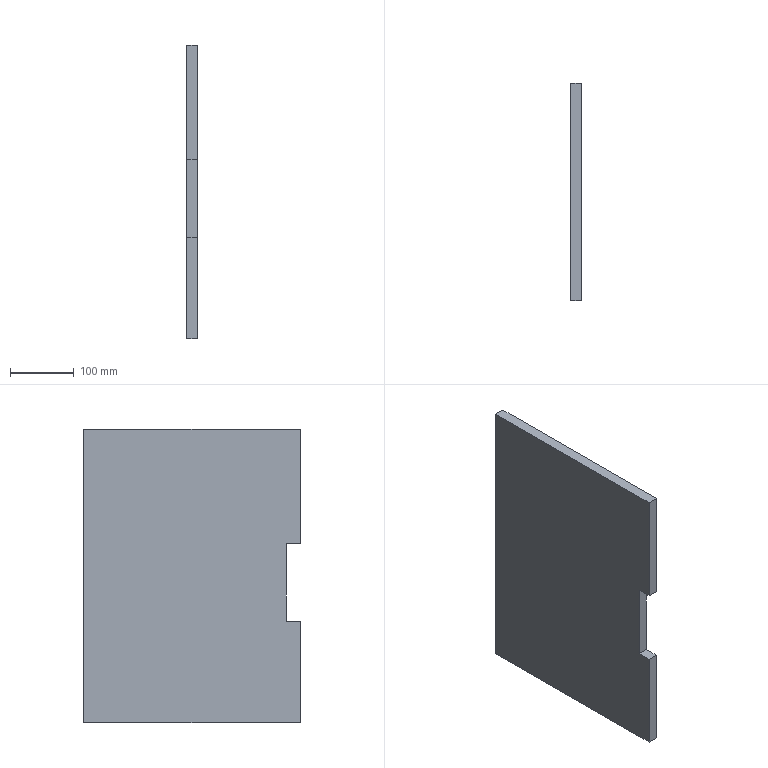Part | SolidWorks | features BaseBody 1 | 1 solid | 10 faces | box 16 x 340 x 460 mm | volume 2459456 mm3 | plane 10
STEP:
#1=CARTESIAN_POINT('',(16.,0.,-71.));
#2=VERTEX_POINT('',#1);
#3=CARTESIAN_POINT('',(16.,22.,-71.));
#4=VERTEX_POINT('',#3);
#5=CARTESIAN_POINT('',(16.,0.,-71.));
#6=DIRECTION('',(0.,1.,0.));
#7=VECTOR('',#6,1000.);
#8=LINE('',#5,#7);
#9=EDGE_CURVE('',#2,#4,#8,.T.);
#10=ORIENTED_EDGE('',*,*,#9,.F.);
#11=CARTESIAN_POINT('',(16.,0.,-230.));
#12=VERTEX_POINT('',#11);
#13=CARTESIAN_POINT('',(16.,0.,0.));
#14=DIRECTION('',(0.,0.,1.));
#15=VECTOR('',#14,1000.);
#16=LINE('',#13,#15);
#17=EDGE_CURVE('',#12,#2,#16,.T.);
#18=ORIENTED_EDGE('',*,*,#17,.F.);
#19=CARTESIAN_POINT('',(16.,340.,-230.));
#20=VERTEX_POINT('',#19);
#21=CARTESIAN_POINT('',(16.,0.,-230.));
#22=DIRECTION('',(0.,-1.,0.));
#23=VECTOR('',#22,1000.);
#24=LINE('',#21,#23);
#25=EDGE_CURVE('',#20,#12,#24,.T.);
#26=ORIENTED_EDGE('',*,*,#25,.F.);
#27=CARTESIAN_POINT('',(16.,340.,230.));
#28=VERTEX_POINT('',#27);
#29=CARTESIAN_POINT('',(16.,340.,0.));
#30=DIRECTION('',(0.,0.,-1.));
#31=VECTOR('',#30,1000.);
#32=LINE('',#29,#31);
#33=EDGE_CURVE('',#28,#20,#32,.T.);
#34=ORIENTED_EDGE('',*,*,#33,.F.);
#35=CARTESIAN_POINT('',(16.,0.,230.));
#36=VERTEX_POINT('',#35);
#37=CARTESIAN_POINT('',(16.,0.,230.));
#38=DIRECTION('',(0.,1.,0.));
#39=VECTOR('',#38,1000.);
#40=LINE('',#37,#39);
#41=EDGE_CURVE('',#36,#28,#40,.T.);
#42=ORIENTED_EDGE('',*,*,#41,.F.);
#43=CARTESIAN_POINT('',(16.,0.,51.));
#44=VERTEX_POINT('',#43);
#45=CARTESIAN_POINT('',(16.,0.,0.));
#46=DIRECTION('',(0.,0.,1.));
#47=VECTOR('',#46,1000.);
#48=LINE('',#45,#47);
#49=EDGE_CURVE('',#44,#36,#48,.T.);
#50=ORIENTED_EDGE('',*,*,#49,.F.);
#51=CARTESIAN_POINT('',(16.,22.,51.));
#52=VERTEX_POINT('',#51);
#53=CARTESIAN_POINT('',(16.,0.,51.));
#54=DIRECTION('',(0.,-1.,0.));
#55=VECTOR('',#54,1000.);
#56=LINE('',#53,#55);
#57=EDGE_CURVE('',#52,#44,#56,.T.);
#58=ORIENTED_EDGE('',*,*,#57,.F.);
#59=CARTESIAN_POINT('',(16.,22.,0.));
#60=DIRECTION('',(0.,0.,1.));
#61=VECTOR('',#60,1000.);
#62=LINE('',#59,#61);
#63=EDGE_CURVE('',#4,#52,#62,.T.);
#64=ORIENTED_EDGE('',*,*,#63,.F.);
#65=EDGE_LOOP('',(#10,#18,#26,#34,#42,#50,#58,#64));
#66=FACE_OUTER_BOUND('',#65,.T.);
#67=CARTESIAN_POINT('',(16.,0.,0.));
#68=DIRECTION('',(-1.,0.,0.));
#69=DIRECTION('',(0.,0.,1.));
#70=AXIS2_PLACEMENT_3D('',#67,#68,#69);
#71=PLANE('',#70);
#72=ADVANCED_FACE('',(#66),#71,.F.);
#73=CARTESIAN_POINT('',(0.,22.,51.));
#74=VERTEX_POINT('',#73);
#75=CARTESIAN_POINT('',(0.,22.,51.));
#76=DIRECTION('',(1.,0.,0.));
#77=VECTOR('',#76,1000.);
#78=LINE('',#75,#77);
#79=EDGE_CURVE('',#74,#52,#78,.T.);
#80=ORIENTED_EDGE('',*,*,#79,.F.);
#81=CARTESIAN_POINT('',(0.,22.,-71.));
#82=VERTEX_POINT('',#81);
#83=CARTESIAN_POINT('',(0.,22.,-71.));
#84=DIRECTION('',(0.,0.,1.));
#85=VECTOR('',#84,1000.);
#86=LINE('',#83,#85);
#87=EDGE_CURVE('',#82,#74,#86,.T.);
#88=ORIENTED_EDGE('',*,*,#87,.F.);
#89=CARTESIAN_POINT('',(0.,22.,-71.));
#90=DIRECTION('',(-1.,0.,0.));
#91=VECTOR('',#90,1000.);
#92=LINE('',#89,#91);
#93=EDGE_CURVE('',#4,#82,#92,.T.);
#94=ORIENTED_EDGE('',*,*,#93,.F.);
#95=ORIENTED_EDGE('',*,*,#63,.T.);
#96=EDGE_LOOP('',(#80,#88,#94,#95));
#97=FACE_OUTER_BOUND('',#96,.T.);
#98=CARTESIAN_POINT('',(0.,22.,-71.));
#99=DIRECTION('',(0.,1.,0.));
#100=DIRECTION('',(0.,0.,1.));
#101=AXIS2_PLACEMENT_3D('',#98,#99,#100);
#102=PLANE('',#101);
#103=ADVANCED_FACE('',(#97),#102,.F.);
#104=ORIENTED_EDGE('',*,*,#93,.T.);
#105=CARTESIAN_POINT('',(0.,0.,-71.));
#106=VERTEX_POINT('',#105);
#107=CARTESIAN_POINT('',(0.,0.,-71.));
#108=DIRECTION('',(0.,1.,0.));
#109=VECTOR('',#108,1000.);
#110=LINE('',#107,#109);
#111=EDGE_CURVE('',#106,#82,#110,.T.);
#112=ORIENTED_EDGE('',*,*,#111,.F.);
#113=CARTESIAN_POINT('',(0.,0.,-71.));
#114=DIRECTION('',(-1.,0.,0.));
#115=VECTOR('',#114,1000.);
#116=LINE('',#113,#115);
#117=EDGE_CURVE('',#2,#106,#116,.T.);
#118=ORIENTED_EDGE('',*,*,#117,.F.);
#119=ORIENTED_EDGE('',*,*,#9,.T.);
#120=EDGE_LOOP('',(#104,#112,#118,#119));
#121=FACE_OUTER_BOUND('',#120,.T.);
#122=CARTESIAN_POINT('',(0.,0.,-71.));
#123=DIRECTION('',(0.,0.,-1.));
#124=DIRECTION('',(0.,1.,0.));
#125=AXIS2_PLACEMENT_3D('',#122,#123,#124);
#126=PLANE('',#125);
#127=ADVANCED_FACE('',(#121),#126,.F.);
#128=ORIENTED_EDGE('',*,*,#117,.T.);
#129=CARTESIAN_POINT('',(0.,0.,-230.));
#130=VERTEX_POINT('',#129);
#131=CARTESIAN_POINT('',(0.,0.,230.));
#132=DIRECTION('',(0.,0.,1.));
#133=VECTOR('',#132,1000.);
#134=LINE('',#131,#133);
#135=EDGE_CURVE('',#130,#106,#134,.T.);
#136=ORIENTED_EDGE('',*,*,#135,.F.);
#137=CARTESIAN_POINT('',(16.,0.,-230.));
#138=DIRECTION('',(-1.,0.,0.));
#139=VECTOR('',#138,1000.);
#140=LINE('',#137,#139);
#141=EDGE_CURVE('',#12,#130,#140,.T.);
#142=ORIENTED_EDGE('',*,*,#141,.F.);
#143=ORIENTED_EDGE('',*,*,#17,.T.);
#144=EDGE_LOOP('',(#128,#136,#142,#143));
#145=FACE_OUTER_BOUND('',#144,.T.);
#146=CARTESIAN_POINT('',(16.,0.,230.));
#147=DIRECTION('',(0.,1.,0.));
#148=DIRECTION('',(0.,0.,1.));
#149=AXIS2_PLACEMENT_3D('',#146,#147,#148);
#150=PLANE('',#149);
#151=ADVANCED_FACE('',(#145),#150,.F.);
#152=CARTESIAN_POINT('',(0.,340.,-230.));
#153=VERTEX_POINT('',#152);
#154=CARTESIAN_POINT('',(16.,340.,-230.));
#155=DIRECTION('',(-1.,0.,0.));
#156=VECTOR('',#155,1000.);
#157=LINE('',#154,#156);
#158=EDGE_CURVE('',#20,#153,#157,.T.);
#159=ORIENTED_EDGE('',*,*,#158,.F.);
#160=ORIENTED_EDGE('',*,*,#25,.T.);
#161=ORIENTED_EDGE('',*,*,#141,.T.);
#162=CARTESIAN_POINT('',(0.,340.,-230.));
#163=DIRECTION('',(0.,-1.,0.));
#164=VECTOR('',#163,1000.);
#165=LINE('',#162,#164);
#166=EDGE_CURVE('',#153,#130,#165,.T.);
#167=ORIENTED_EDGE('',*,*,#166,.F.);
#168=EDGE_LOOP('',(#159,#160,#161,#167));
#169=FACE_OUTER_BOUND('',#168,.T.);
#170=CARTESIAN_POINT('',(16.,340.,-230.));
#171=DIRECTION('',(0.,0.,1.));
#172=DIRECTION('',(0.,-1.,0.));
#173=AXIS2_PLACEMENT_3D('',#170,#171,#172);
#174=PLANE('',#173);
#175=ADVANCED_FACE('',(#169),#174,.F.);
#176=CARTESIAN_POINT('',(0.,340.,230.));
#177=VERTEX_POINT('',#176);
#178=CARTESIAN_POINT('',(16.,340.,230.));
#179=DIRECTION('',(-1.,0.,0.));
#180=VECTOR('',#179,1000.);
#181=LINE('',#178,#180);
#182=EDGE_CURVE('',#28,#177,#181,.T.);
#183=ORIENTED_EDGE('',*,*,#182,.F.);
#184=ORIENTED_EDGE('',*,*,#33,.T.);
#185=ORIENTED_EDGE('',*,*,#158,.T.);
#186=CARTESIAN_POINT('',(0.,340.,230.));
#187=DIRECTION('',(0.,0.,-1.));
#188=VECTOR('',#187,1000.);
#189=LINE('',#186,#188);
#190=EDGE_CURVE('',#177,#153,#189,.T.);
#191=ORIENTED_EDGE('',*,*,#190,.F.);
#192=EDGE_LOOP('',(#183,#184,#185,#191));
#193=FACE_OUTER_BOUND('',#192,.T.);
#194=CARTESIAN_POINT('',(16.,340.,230.));
#195=DIRECTION('',(0.,-1.,0.));
#196=DIRECTION('',(0.,0.,-1.));
#197=AXIS2_PLACEMENT_3D('',#194,#195,#196);
#198=PLANE('',#197);
#199=ADVANCED_FACE('',(#193),#198,.F.);
#200=CARTESIAN_POINT('',(0.,0.,230.));
#201=VERTEX_POINT('',#200);
#202=CARTESIAN_POINT('',(16.,0.,230.));
#203=DIRECTION('',(-1.,0.,0.));
#204=VECTOR('',#203,1000.);
#205=LINE('',#202,#204);
#206=EDGE_CURVE('',#36,#201,#205,.T.);
#207=ORIENTED_EDGE('',*,*,#206,.F.);
#208=ORIENTED_EDGE('',*,*,#41,.T.);
#209=ORIENTED_EDGE('',*,*,#182,.T.);
#210=CARTESIAN_POINT('',(0.,0.,230.));
#211=DIRECTION('',(0.,1.,0.));
#212=VECTOR('',#211,1000.);
#213=LINE('',#210,#212);
#214=EDGE_CURVE('',#201,#177,#213,.T.);
#215=ORIENTED_EDGE('',*,*,#214,.F.);
#216=EDGE_LOOP('',(#207,#208,#209,#215));
#217=FACE_OUTER_BOUND('',#216,.T.);
#218=CARTESIAN_POINT('',(16.,0.,230.));
#219=DIRECTION('',(0.,0.,-1.));
#220=DIRECTION('',(0.,1.,0.));
#221=AXIS2_PLACEMENT_3D('',#218,#219,#220);
#222=PLANE('',#221);
#223=ADVANCED_FACE('',(#217),#222,.F.);
#224=CARTESIAN_POINT('',(0.,0.,51.));
#225=VERTEX_POINT('',#224);
#226=CARTESIAN_POINT('',(16.,0.,51.));
#227=DIRECTION('',(-1.,0.,0.));
#228=VECTOR('',#227,1000.);
#229=LINE('',#226,#228);
#230=EDGE_CURVE('',#44,#225,#229,.T.);
#231=ORIENTED_EDGE('',*,*,#230,.F.);
#232=ORIENTED_EDGE('',*,*,#49,.T.);
#233=ORIENTED_EDGE('',*,*,#206,.T.);
#234=CARTESIAN_POINT('',(0.,0.,230.));
#235=DIRECTION('',(0.,0.,1.));
#236=VECTOR('',#235,1000.);
#237=LINE('',#234,#236);
#238=EDGE_CURVE('',#225,#201,#237,.T.);
#239=ORIENTED_EDGE('',*,*,#238,.F.);
#240=EDGE_LOOP('',(#231,#232,#233,#239));
#241=FACE_OUTER_BOUND('',#240,.T.);
#242=CARTESIAN_POINT('',(16.,0.,230.));
#243=DIRECTION('',(0.,1.,0.));
#244=DIRECTION('',(0.,0.,1.));
#245=AXIS2_PLACEMENT_3D('',#242,#243,#244);
#246=PLANE('',#245);
#247=ADVANCED_FACE('',(#241),#246,.F.);
#248=ORIENTED_EDGE('',*,*,#230,.T.);
#249=CARTESIAN_POINT('',(0.,0.,51.));
#250=DIRECTION('',(0.,-1.,0.));
#251=VECTOR('',#250,1000.);
#252=LINE('',#249,#251);
#253=EDGE_CURVE('',#74,#225,#252,.T.);
#254=ORIENTED_EDGE('',*,*,#253,.F.);
#255=ORIENTED_EDGE('',*,*,#79,.T.);
#256=ORIENTED_EDGE('',*,*,#57,.T.);
#257=EDGE_LOOP('',(#248,#254,#255,#256));
#258=FACE_OUTER_BOUND('',#257,.T.);
#259=CARTESIAN_POINT('',(0.,0.,51.));
#260=DIRECTION('',(0.,0.,1.));
#261=DIRECTION('',(0.,-1.,0.));
#262=AXIS2_PLACEMENT_3D('',#259,#260,#261);
#263=PLANE('',#262);
#264=ADVANCED_FACE('',(#258),#263,.F.);
#265=ORIENTED_EDGE('',*,*,#166,.T.);
#266=ORIENTED_EDGE('',*,*,#135,.T.);
#267=ORIENTED_EDGE('',*,*,#111,.T.);
#268=ORIENTED_EDGE('',*,*,#87,.T.);
#269=ORIENTED_EDGE('',*,*,#253,.T.);
#270=ORIENTED_EDGE('',*,*,#238,.T.);
#271=ORIENTED_EDGE('',*,*,#214,.T.);
#272=ORIENTED_EDGE('',*,*,#190,.T.);
#273=EDGE_LOOP('',(#265,#266,#267,#268,#269,#270,#271,#272));
#274=FACE_OUTER_BOUND('',#273,.T.);
#275=CARTESIAN_POINT('',(0.,0.,0.));
#276=DIRECTION('',(-1.,0.,0.));
#277=DIRECTION('',(0.,0.,1.));
#278=AXIS2_PLACEMENT_3D('',#275,#276,#277);
#279=PLANE('',#278);
#280=ADVANCED_FACE('',(#274),#279,.T.);
#281=CLOSED_SHELL('',(#72,#103,#127,#151,#175,#199,#223,#247,#264,#280));
#282=MANIFOLD_SOLID_BREP('',#281);
#283=CARTESIAN_POINT('',(0.,0.,0.));
#284=DIRECTION('',(0.,0.,1.));
#285=DIRECTION('',(1.,0.,0.));
#286=AXIS2_PLACEMENT_3D('',#283,#284,#285);
#287=(LENGTH_UNIT()NAMED_UNIT(*)SI_UNIT(.MILLI.,.METRE.));
#288=UNCERTAINTY_MEASURE_WITH_UNIT(LENGTH_MEASURE(0.00001),#287,'','');
#289=(NAMED_UNIT(*)PLANE_ANGLE_UNIT()SI_UNIT($,.RADIAN.));
#290=(NAMED_UNIT(*)SI_UNIT($,.STERADIAN.)SOLID_ANGLE_UNIT());
#291=(GEOMETRIC_REPRESENTATION_CONTEXT(3)GLOBAL_UNCERTAINTY_ASSIGNED_CONTEXT((#288))GLOBAL_UNIT_ASSIGNED_CONTEXT((#287,#289,#290))REPRESENTATION_CONTEXT('',''));
#292=ADVANCED_BREP_SHAPE_REPRESENTATION('',(#282,#286),#291);